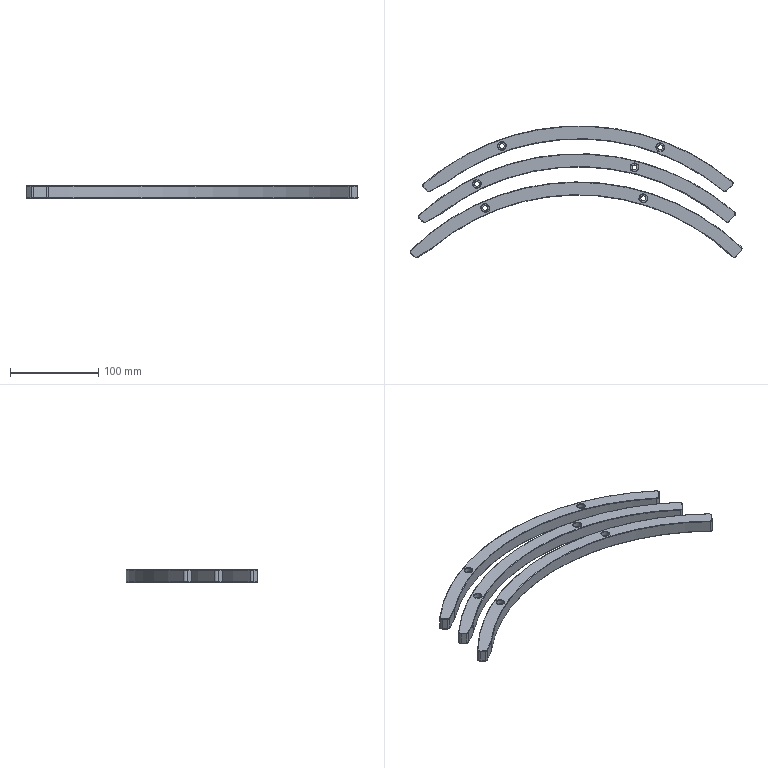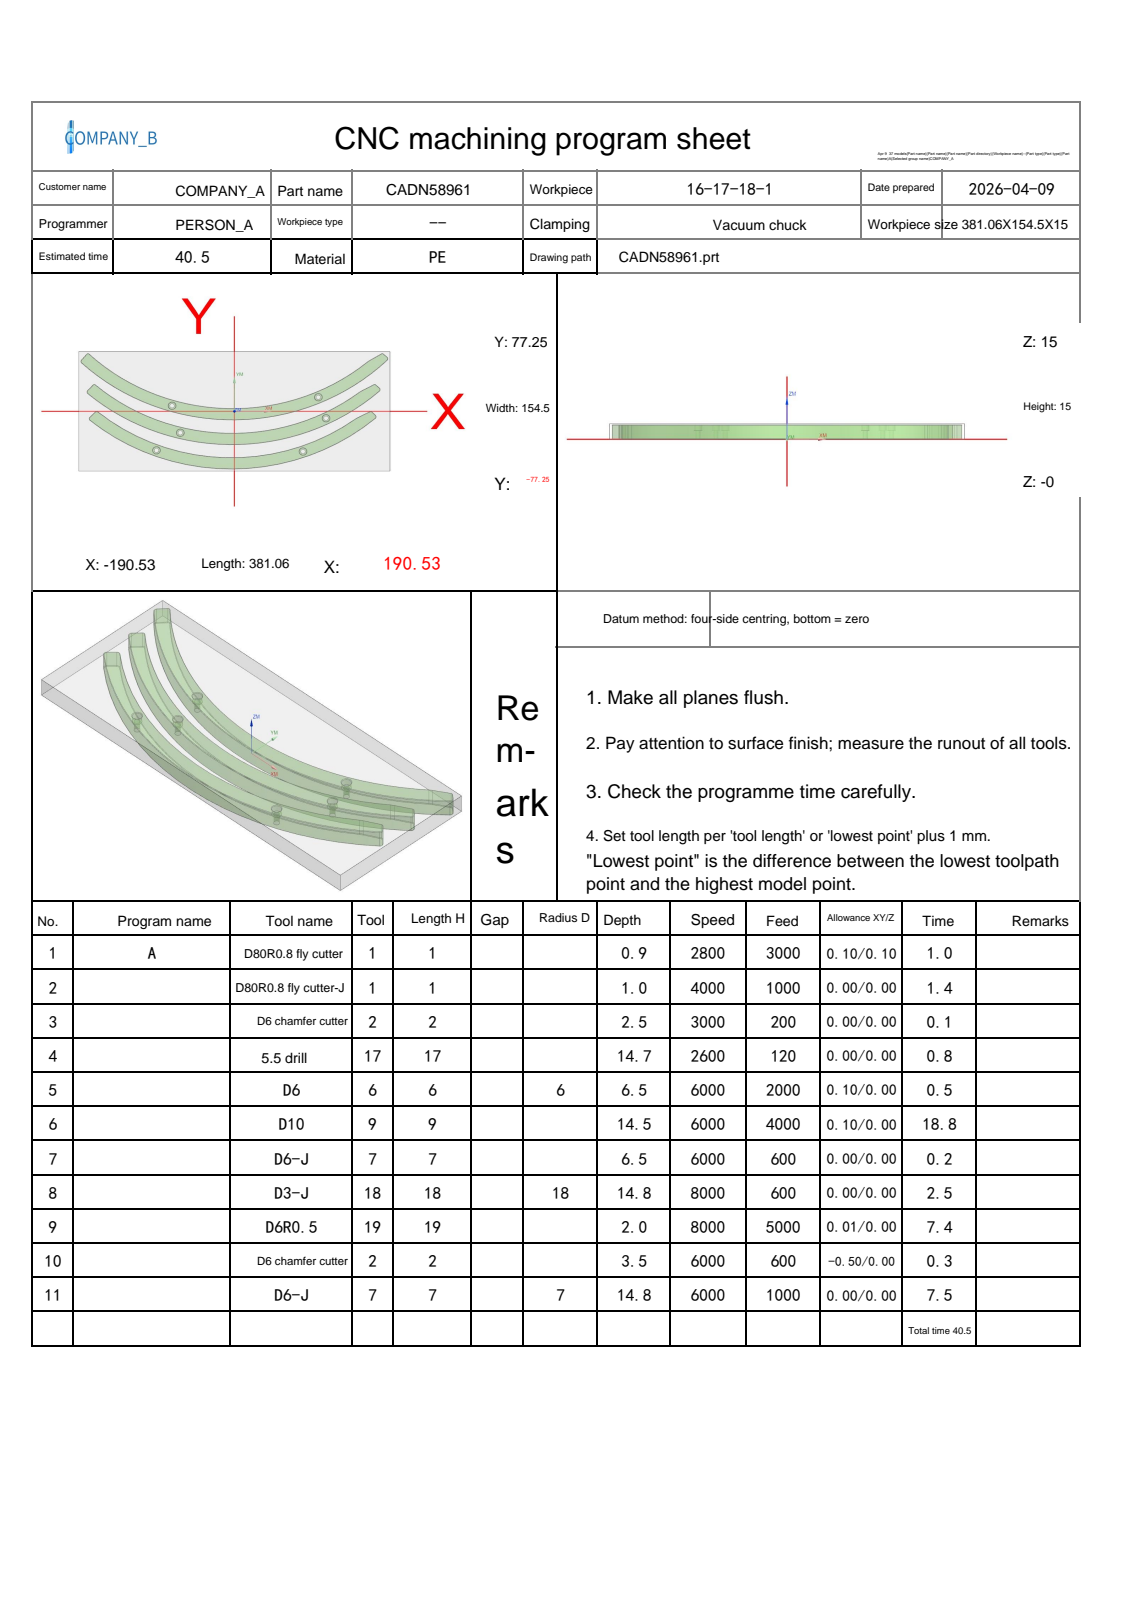NC program | NX | posted by the shop | part box 376.065 x 149.521 x 14 mm
Lines 1 to 356 of 3929:
%
O0001
(Machine time: 42.57 MIN)
(===Total Tool:8===)
(T1=D80R0.8 fly cutter D=80.  R=0.8  D-  H01 Z=14.   )
(T2=D6 chamfer cutter   D=6.   R=0.   D-  H02 Z=11.5  )
(T17=5.5 drill  D=5.5  DR_a=118 D-  H17 Z=0.3   )
(T6=D6      D=6.   R=0.   D6  H06 Z=8.5   )
(T9=D10     D=10.  R=0.   D-  H09 Z=0.5   )
(T7=D6-J    D=6.   R=0.   D-  H07 Z=0.2   )
(T18=D3-J   D=3.   R=0.   D18 H18 Z=0.2   )
(T19=D6R0.5 D=6.   R=0.5  D-  H19 Z=13.   )
G80 G90 G17 G49 G40
G91 G28 Z0
M01
N1 T01 M06
(D80R0.8 fly cutter  D=80. R=0.8 H=01 ce=0.10 di=0.10)
(MAX_Z=34. MIN_Z=14.1 Time=0.97M)
G00 G90 G54 X204.139 Y-50.867 M03 S2800
G43 H01 Z34.
M08
Z16.55
G01 Z14.55 F3000.
X185.004 Y-50.865
X-189.58 Y-50.833
G02 X-194.507 Y-49.132 I.005 J8.
G01 X-197.443 Y-46.831
X-197.573 Y-46.726
X-202.559 Y-42.645
X-202.629 Y-42.587
G02 X-217.851 Y-13.587 I27.686 J33.028
G01 X-217.866 Y-13.403
X-218.01 Y-11.355
G02 X-218.028 Y-10.854 I7.183 J.501
X-210.831 Y-3.654 I7.2 J0.0
G01 X207.91 Y-3.691
G03 X215.768 Y2.828 I-.003 J8.
G01 X221.985 Y35.903
G03 X222.095 Y37.085 I-6.29 J1.182
X215.695 Y43.485 I-6.4 J0.0
G01 X-224.849 Y43.523
X-237.059 Y43.524
Z16.55
G00 X204.139 Y-50.867
Z16.1
G01 Z14.1
X185.004 Y-50.865
X-189.58 Y-50.833
G02 X-194.507 Y-49.132 I.005 J8.
G01 X-197.443 Y-46.831
X-197.573 Y-46.726
X-202.559 Y-42.645
X-202.629 Y-42.587
G02 X-217.851 Y-13.587 I27.686 J33.028
G01 X-217.866 Y-13.403
X-218.01 Y-11.355
G02 X-218.028 Y-10.854 I7.183 J.501
X-210.831 Y-3.654 I7.2 J0.0
G01 X207.91 Y-3.691
G03 X215.768 Y2.828 I-.003 J8.
G01 X221.985 Y35.903
G03 X222.095 Y37.085 I-6.29 J1.182
X215.695 Y43.485 I-6.4 J0.0
G01 X-224.849 Y43.523
X-237.059 Y43.524
Z16.1
G00 Z34.
G91 G28 Z0.0
M05
M09
G91 G28 Z0.0
M01
N2 T01 M06
(D80R0.8 fly cutter-J  D=80. R=0.8 H=01 ce=0.00 di=0.00)
(MAX_Z=34. MIN_Z=14. Time=1.42M)
G00 G90 G54 X204.1 Y-50.771 M03 S4000
G43 H01 Z34.
M08
Z16.
G01 Z14. F1000.
X184.968 Y-50.769
X-189.564 Y-50.733
G02 X-194.469 Y-49.049 I.005 J8.
G01 X-195.709 Y-48.085
X-195.795 Y-48.016
X-199.117 Y-45.355
X-199.202 Y-45.286
X-202.508 Y-42.56
X-202.554 Y-42.522
G02 X-217.854 Y-12.312 I27.611 J32.963
G01 X-217.856 Y-12.272
X-217.921 Y-11.348
G02 X-217.938 Y-10.852 I7.183 J.496
X-210.741 Y-3.652 I7.2 J0.0
G01 X207.808 Y-3.692
G03 X215.671 Y2.832 I0.0 J8.
G01 X221.865 Y35.806
G03 X221.975 Y36.987 I-6.29 J1.181
X215.575 Y43.387 I-6.4 J0.0
G01 X-224.734 Y43.429
X-236.945 Y43.43
Z16.
G00 Z34.
G91 G28 Z0.0
M05
M09
G91 G28 Z0.0
M01
N3 T02 M06
(D6 chamfer cutter  D=6. R=0. H=02 ce=0.00 di=0.00)
(MAX_Z=34. MIN_Z=12.5 Time=0.11M)
G00 G90 G54 X-95.398 Y-50.438 M03 S3000
G43 H02 Z34.
M08
G98 G81 X-95.398 Y-50.438 Z12.5 R15. F200.
X-66.222 Y-27.703
X-76.256 Y7.232
X83.992 Y-51.936
X112.192 Y-8.961
X102.803 Y18.225
G80
G00 Z34.
G91 G28 Z0.0
M05
M09
G91 G28 Z0.0
M01
N4 T17 M06
(5.5 drill D=5.5 DR_a=118 H=17)
(MAX_Z=34. MIN_Z=0.3 Time=0.77M)
G00 G90 G54 X-95.398 Y-50.438 M03 S2600
G43 H17 Z34.
M08
G98 G83 X-95.398 Y-50.438 Z.3 R15. F120. Q3.
X-66.222 Y-27.703
X-76.256 Y7.232
X83.992 Y-51.936
X112.192 Y-8.961
X102.803 Y18.225
G80
G00 Z34.
G91 G28 Z0.0
M05
M09
G91 G28 Z0.0
M01
N5 T06 M06
(D6  D=6. R=0. H=06 ce=0.10 di=0.00)
(D.N=06 MAX_Z=34. MIN_Z=8.5 Time=0.52M)
G00 G90 G54 X112.192 Y-8.961 M03 S6000
G43 H06 Z34.
M08
Z14.3
G41 D06
G01 X112.196 Y-8.861 F2000.
G03 X111.498 Y-8.256 I-.698 J-.1
X110.792 Y-8.961 I0.0 J-.705
X110.792 Y-8.961 Z13.95 I1.4 J0.0
X110.792 Y-8.961 Z13.6 I1.4 J0.0
X110.792 Y-8.961 Z13.25 I1.4 J0.0
X110.792 Y-8.961 Z12.9 I1.4 J0.0
X110.792 Y-8.961 Z12.55 I1.4 J0.0
X110.792 Y-8.961 Z12.2 I1.4 J0.0
X110.792 Y-8.961 Z11.85 I1.4 J0.0
X110.792 Y-8.961 Z11.5 I1.4 J0.0
X110.792 Y-8.961 Z11.15 I1.4 J0.0
X110.792 Y-8.961 Z10.8 I1.4 J0.0
X110.792 Y-8.961 Z10.45 I1.4 J0.0
X110.792 Y-8.961 Z10.1 I1.4 J0.0
X110.792 Y-8.961 Z9.75 I1.4 J0.0
X110.792 Y-8.961 Z9.4 I1.4 J0.0
X110.792 Y-8.961 Z9.05 I1.4 J0.0
X110.792 Y-8.961 Z8.7 I1.4 J0.0
X113.454 Y-8.354 Z8.5 I1.4 J0.0
X112.192 Y-7.561 I-1.261 J-.607
X110.792 Y-8.961 I0.0 J-1.4
X112.192 Y-10.361 I1.4 J0.0
X113.592 Y-8.961 I0.0 J1.4
X113.454 Y-8.354 I-1.4 J0.0
X112.818 Y-7.955 I-.635 J-.306
X112.113 Y-8.66 I0.0 J-.705
X112.146 Y-8.873 I.705 J0.0
G01 G40 X112.192 Y-8.961
G00 Z34.
X102.803 Y18.225
Z14.3
G41 D06
G01 X102.807 Y18.325
G03 X102.109 Y18.931 I-.698 J-.1
X101.403 Y18.225 I0.0 J-.705
X101.403 Y18.225 Z13.95 I1.4 J0.0
X101.403 Y18.225 Z13.6 I1.4 J0.0
X101.403 Y18.225 Z13.25 I1.4 J0.0
X101.403 Y18.225 Z12.9 I1.4 J0.0
X101.403 Y18.225 Z12.55 I1.4 J0.0
X101.403 Y18.225 Z12.2 I1.4 J0.0
X101.403 Y18.225 Z11.85 I1.4 J0.0
X101.403 Y18.225 Z11.5 I1.4 J0.0
X101.403 Y18.225 Z11.15 I1.4 J0.0
X101.403 Y18.225 Z10.8 I1.4 J0.0
X101.403 Y18.225 Z10.45 I1.4 J0.0
X101.403 Y18.225 Z10.1 I1.4 J0.0
X101.403 Y18.225 Z9.75 I1.4 J0.0
X101.403 Y18.225 Z9.4 I1.4 J0.0
X101.403 Y18.225 Z9.05 I1.4 J0.0
X101.403 Y18.225 Z8.7 I1.4 J0.0
X104.065 Y18.833 Z8.5 I1.4 J0.0
X102.803 Y19.625 I-1.261 J-.607
X101.403 Y18.225 I0.0 J-1.4
X102.803 Y16.825 I1.4 J0.0
X104.203 Y18.225 I0.0 J1.4
X104.065 Y18.833 I-1.4 J0.0
X103.429 Y19.232 I-.635 J-.306
X102.724 Y18.527 I0.0 J-.705
X102.757 Y18.314 I.705 J0.0
G01 G40 X102.803 Y18.225
G00 Z34.
X83.992 Y-51.936
Z14.3
G41 D06
G01 X83.995 Y-51.836
G03 X83.297 Y-51.231 I-.698 J-.1
X82.592 Y-51.936 I0.0 J-.705
X82.592 Y-51.936 Z13.95 I1.4 J0.0
X82.592 Y-51.936 Z13.6 I1.4 J0.0
X82.592 Y-51.936 Z13.25 I1.4 J0.0
X82.592 Y-51.936 Z12.9 I1.4 J0.0
X82.592 Y-51.936 Z12.55 I1.4 J0.0
X82.592 Y-51.936 Z12.2 I1.4 J0.0
X82.592 Y-51.936 Z11.85 I1.4 J0.0
X82.592 Y-51.936 Z11.5 I1.4 J0.0
X82.592 Y-51.936 Z11.15 I1.4 J0.0
X82.592 Y-51.936 Z10.8 I1.4 J0.0
X82.592 Y-51.936 Z10.45 I1.4 J0.0
X82.592 Y-51.936 Z10.1 I1.4 J0.0
X82.592 Y-51.936 Z9.75 I1.4 J0.0
X82.592 Y-51.936 Z9.4 I1.4 J0.0
X82.592 Y-51.936 Z9.05 I1.4 J0.0
X82.592 Y-51.936 Z8.7 I1.4 J0.0
X85.253 Y-51.329 Z8.5 I1.4 J0.0
X83.992 Y-50.536 I-1.261 J-.607
X82.592 Y-51.936 I0.0 J-1.4
X83.992 Y-53.336 I1.4 J0.0
X85.392 Y-51.936 I0.0 J1.4
X85.253 Y-51.329 I-1.4 J0.0
X84.618 Y-50.929 I-.635 J-.306
X83.912 Y-51.635 I0.0 J-.705
X83.945 Y-51.847 I.705 J0.0
G01 G40 X83.992 Y-51.936
G00 Z34.
X-76.256 Y7.232
Z14.3
G41 D06
G01 X-76.252 Y7.332
G03 X-76.95 Y7.937 I-.698 J-.1
X-77.656 Y7.232 I0.0 J-.705
X-77.656 Y7.232 Z13.95 I1.4 J0.0
X-77.656 Y7.232 Z13.6 I1.4 J0.0
X-77.656 Y7.232 Z13.25 I1.4 J0.0
X-77.656 Y7.232 Z12.9 I1.4 J0.0
X-77.656 Y7.232 Z12.55 I1.4 J0.0
X-77.656 Y7.232 Z12.2 I1.4 J0.0
X-77.656 Y7.232 Z11.85 I1.4 J0.0
X-77.656 Y7.232 Z11.5 I1.4 J0.0
X-77.656 Y7.232 Z11.15 I1.4 J0.0
X-77.656 Y7.232 Z10.8 I1.4 J0.0
X-77.656 Y7.232 Z10.45 I1.4 J0.0
X-77.656 Y7.232 Z10.1 I1.4 J0.0
X-77.656 Y7.232 Z9.75 I1.4 J0.0
X-77.656 Y7.232 Z9.4 I1.4 J0.0
X-77.656 Y7.232 Z9.05 I1.4 J0.0
X-77.656 Y7.232 Z8.7 I1.4 J0.0
X-74.994 Y7.839 Z8.5 I1.4 J0.0
X-76.256 Y8.632 I-1.261 J-.607
X-77.656 Y7.232 I0.0 J-1.4
X-76.256 Y5.832 I1.4 J0.0
X-74.856 Y7.232 I0.0 J1.4
X-74.994 Y7.839 I-1.4 J0.0
X-75.63 Y8.238 I-.635 J-.306
X-76.335 Y7.533 I0.0 J-.705
X-76.302 Y7.32 I.705 J0.0
G01 G40 X-76.256 Y7.232
G00 Z34.
X-66.222 Y-27.703
Z14.3
G41 D06
G01 X-66.219 Y-27.603
G03 X-66.917 Y-26.998 I-.698 J-.1
X-67.622 Y-27.703 I0.0 J-.705
X-67.622 Y-27.703 Z13.95 I1.4 J0.0
X-67.622 Y-27.703 Z13.6 I1.4 J0.0
X-67.622 Y-27.703 Z13.25 I1.4 J0.0
X-67.622 Y-27.703 Z12.9 I1.4 J0.0
X-67.622 Y-27.703 Z12.55 I1.4 J0.0
X-67.622 Y-27.703 Z12.2 I1.4 J0.0
X-67.622 Y-27.703 Z11.85 I1.4 J0.0
X-67.622 Y-27.703 Z11.5 I1.4 J0.0
X-67.622 Y-27.703 Z11.15 I1.4 J0.0
X-67.622 Y-27.703 Z10.8 I1.4 J0.0
X-67.622 Y-27.703 Z10.45 I1.4 J0.0
X-67.622 Y-27.703 Z10.1 I1.4 J0.0
X-67.622 Y-27.703 Z9.75 I1.4 J0.0
X-67.622 Y-27.703 Z9.4 I1.4 J0.0
X-67.622 Y-27.703 Z9.05 I1.4 J0.0
X-67.622 Y-27.703 Z8.7 I1.4 J0.0
X-64.961 Y-27.096 Z8.5 I1.4 J0.0
X-66.222 Y-26.303 I-1.261 J-.607
X-67.622 Y-27.703 I0.0 J-1.4
X-66.222 Y-29.103 I1.4 J0.0
X-64.822 Y-27.703 I0.0 J1.4
X-64.961 Y-27.096 I-1.4 J0.0
X-65.596 Y-26.697 I-.635 J-.306
X-66.301 Y-27.402 I0.0 J-.705
X-66.268 Y-27.614 I.705 J0.0
G01 G40 X-66.222 Y-27.703
G00 Z34.
X-95.398 Y-50.438
Z14.3
G41 D06
G01 X-95.395 Y-50.338
G03 X-96.093 Y-49.732 I-.698 J-.1
X-96.798 Y-50.437 I0.0 J-.705
X-96.798 Y-50.437 Z13.95 I1.4 J0.0
X-96.798 Y-50.437 Z13.6 I1.4 J0.0
X-96.798 Y-50.437 Z13.25 I1.4 J0.0
X-96.798 Y-50.437 Z12.9 I1.4 J0.0
X-96.798 Y-50.437 Z12.55 I1.4 J0.0
X-96.798 Y-50.437 Z12.2 I1.4 J0.0
X-96.798 Y-50.437 Z11.85 I1.4 J0.0
X-96.798 Y-50.437 Z11.5 I1.4 J0.0
X-96.798 Y-50.437 Z11.15 I1.4 J0.0
X-96.798 Y-50.437 Z10.8 I1.4 J0.0
X-96.798 Y-50.437 Z10.45 I1.4 J0.0
X-96.798 Y-50.437 Z10.1 I1.4 J0.0
X-96.798 Y-50.437 Z9.75 I1.4 J0.0
X-96.798 Y-50.437 Z9.4 I1.4 J0.0
X-96.798 Y-50.437 Z9.05 I1.4 J0.0
X-96.798 Y-50.437 Z8.7 I1.4 J0.0
X-94.137 Y-49.83 Z8.5 I1.4 J0.0
X-95.398 Y-49.038 I-1.261 J-.607
X-96.798 Y-50.438 I0.0 J-1.4
X-95.398 Y-51.838 I1.4 J0.0
X-93.998 Y-50.438 I0.0 J1.4
X-94.137 Y-49.83 I-1.4 J0.0
X-94.772 Y-49.431 I-.635 J-.306
X-95.478 Y-50.136 I0.0 J-.705
X-95.445 Y-50.349 I.705 J0.0
G01 G40 X-95.398 Y-50.438
G00 Z34.
G91 G28 Z0.0
M05
M09
G91 G28 Z0.0
M01